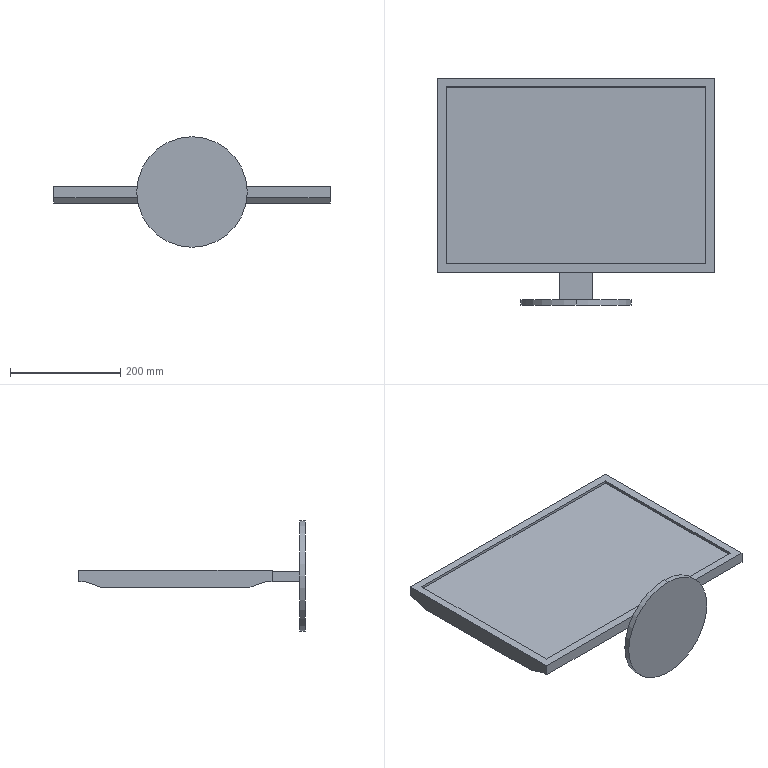Part | SolidWorks | features ICE 4, Extrusion 1 | 1 solid | 22 faces | box 500 x 410 x 200 mm | volume 4616159 mm3 | plane 20 | cylinder 2 | commonest cylinder face diameters 200 x2
STEP:
#1=CARTESIAN_POINT('',(250.,-60.,-90.));
#2=VERTEX_POINT('',#1);
#3=CARTESIAN_POINT('',(250.,-60.,110.));
#4=VERTEX_POINT('',#3);
#5=CARTESIAN_POINT('',(250.,-60.,10.));
#6=DIRECTION('',(0.,-1.,0.));
#7=DIRECTION('',(0.,0.,-1.));
#8=AXIS2_PLACEMENT_3D('',#5,#6,#7);
#9=CIRCLE('',#8,100.);
#10=EDGE_CURVE('',#2,#4,#9,.T.);
#11=ORIENTED_EDGE('',*,*,#10,.F.);
#12=CARTESIAN_POINT('',(250.,-50.,-90.));
#13=VERTEX_POINT('',#12);
#14=CARTESIAN_POINT('',(250.,-60.,-90.));
#15=DIRECTION('',(0.,1.,0.));
#16=VECTOR('',#15,1000.);
#17=LINE('',#14,#16);
#18=EDGE_CURVE('',#2,#13,#17,.T.);
#19=ORIENTED_EDGE('',*,*,#18,.T.);
#20=CARTESIAN_POINT('',(250.,-50.,110.));
#21=VERTEX_POINT('',#20);
#22=CARTESIAN_POINT('',(250.,-50.,10.));
#23=DIRECTION('',(0.,-1.,0.));
#24=DIRECTION('',(0.,0.,-1.));
#25=AXIS2_PLACEMENT_3D('',#22,#23,#24);
#26=CIRCLE('',#25,100.);
#27=EDGE_CURVE('',#13,#21,#26,.T.);
#28=ORIENTED_EDGE('',*,*,#27,.T.);
#29=CARTESIAN_POINT('',(250.,-60.,110.));
#30=DIRECTION('',(0.,1.,0.));
#31=VECTOR('',#30,1000.);
#32=LINE('',#29,#31);
#33=EDGE_CURVE('',#4,#21,#32,.T.);
#34=ORIENTED_EDGE('',*,*,#33,.F.);
#35=EDGE_LOOP('',(#11,#19,#28,#34));
#36=FACE_OUTER_BOUND('',#35,.T.);
#37=CARTESIAN_POINT('',(250.,-60.,10.));
#38=DIRECTION('',(0.,1.,0.));
#39=DIRECTION('',(0.,0.,1.));
#40=AXIS2_PLACEMENT_3D('',#37,#38,#39);
#41=CYLINDRICAL_SURFACE('',#40,100.);
#42=ADVANCED_FACE('',(#36),#41,.T.);
#43=CARTESIAN_POINT('',(280.,0.,0.));
#44=VERTEX_POINT('',#43);
#45=CARTESIAN_POINT('',(280.,0.,18.));
#46=VERTEX_POINT('',#45);
#47=CARTESIAN_POINT('',(280.,0.,18.));
#48=DIRECTION('',(0.,0.,1.));
#49=VECTOR('',#48,1000.);
#50=LINE('',#47,#49);
#51=EDGE_CURVE('',#44,#46,#50,.T.);
#52=ORIENTED_EDGE('',*,*,#51,.F.);
#53=CARTESIAN_POINT('',(500.,0.,0.));
#54=VERTEX_POINT('',#53);
#55=CARTESIAN_POINT('',(0.,0.,0.));
#56=DIRECTION('',(1.,0.,0.));
#57=VECTOR('',#56,1000.);
#58=LINE('',#55,#57);
#59=EDGE_CURVE('',#44,#54,#58,.T.);
#60=ORIENTED_EDGE('',*,*,#59,.T.);
#61=CARTESIAN_POINT('',(500.,0.,20.));
#62=VERTEX_POINT('',#61);
#63=CARTESIAN_POINT('',(500.,0.,20.));
#64=DIRECTION('',(0.,0.,-1.));
#65=VECTOR('',#64,1000.);
#66=LINE('',#63,#65);
#67=EDGE_CURVE('',#62,#54,#66,.T.);
#68=ORIENTED_EDGE('',*,*,#67,.F.);
#69=CARTESIAN_POINT('',(0.,0.,20.));
#70=VERTEX_POINT('',#69);
#71=CARTESIAN_POINT('',(0.,0.,20.));
#72=DIRECTION('',(1.,0.,0.));
#73=VECTOR('',#72,1000.);
#74=LINE('',#71,#73);
#75=EDGE_CURVE('',#70,#62,#74,.T.);
#76=ORIENTED_EDGE('',*,*,#75,.F.);
#77=CARTESIAN_POINT('',(0.,0.,0.));
#78=VERTEX_POINT('',#77);
#79=CARTESIAN_POINT('',(0.,0.,20.));
#80=DIRECTION('',(0.,0.,-1.));
#81=VECTOR('',#80,1000.);
#82=LINE('',#79,#81);
#83=EDGE_CURVE('',#70,#78,#82,.T.);
#84=ORIENTED_EDGE('',*,*,#83,.T.);
#85=CARTESIAN_POINT('',(220.,0.,0.));
#86=VERTEX_POINT('',#85);
#87=CARTESIAN_POINT('',(0.,0.,0.));
#88=DIRECTION('',(1.,0.,0.));
#89=VECTOR('',#88,1000.);
#90=LINE('',#87,#89);
#91=EDGE_CURVE('',#78,#86,#90,.T.);
#92=ORIENTED_EDGE('',*,*,#91,.T.);
#93=CARTESIAN_POINT('',(220.,0.,18.));
#94=VERTEX_POINT('',#93);
#95=CARTESIAN_POINT('',(220.,0.,18.));
#96=DIRECTION('',(0.,0.,-1.));
#97=VECTOR('',#96,1000.);
#98=LINE('',#95,#97);
#99=EDGE_CURVE('',#94,#86,#98,.T.);
#100=ORIENTED_EDGE('',*,*,#99,.F.);
#101=CARTESIAN_POINT('',(220.,0.,18.));
#102=DIRECTION('',(-1.,0.,0.));
#103=VECTOR('',#102,1000.);
#104=LINE('',#101,#103);
#105=EDGE_CURVE('',#46,#94,#104,.T.);
#106=ORIENTED_EDGE('',*,*,#105,.F.);
#107=EDGE_LOOP('',(#52,#60,#68,#76,#84,#92,#100,#106));
#108=FACE_OUTER_BOUND('',#107,.T.);
#109=CARTESIAN_POINT('',(0.,0.,20.));
#110=DIRECTION('',(0.,1.,0.));
#111=DIRECTION('',(0.,0.,1.));
#112=AXIS2_PLACEMENT_3D('',#109,#110,#111);
#113=PLANE('',#112);
#114=ADVANCED_FACE('',(#108),#113,.F.);
#115=CARTESIAN_POINT('',(0.,10.,0.));
#116=VERTEX_POINT('',#115);
#117=CARTESIAN_POINT('',(0.,0.,0.));
#118=DIRECTION('',(0.,-1.,0.));
#119=VECTOR('',#118,1000.);
#120=LINE('',#117,#119);
#121=EDGE_CURVE('',#116,#78,#120,.T.);
#122=ORIENTED_EDGE('',*,*,#121,.F.);
#123=CARTESIAN_POINT('',(500.,10.,0.));
#124=VERTEX_POINT('',#123);
#125=CARTESIAN_POINT('',(0.,10.,0.));
#126=DIRECTION('',(1.,0.,0.));
#127=VECTOR('',#126,1000.);
#128=LINE('',#125,#127);
#129=EDGE_CURVE('',#116,#124,#128,.T.);
#130=ORIENTED_EDGE('',*,*,#129,.T.);
#131=CARTESIAN_POINT('',(500.,0.,0.));
#132=DIRECTION('',(0.,1.,0.));
#133=VECTOR('',#132,1000.);
#134=LINE('',#131,#133);
#135=EDGE_CURVE('',#54,#124,#134,.T.);
#136=ORIENTED_EDGE('',*,*,#135,.F.);
#137=ORIENTED_EDGE('',*,*,#59,.F.);
#138=CARTESIAN_POINT('',(280.,-50.,0.));
#139=VERTEX_POINT('',#138);
#140=CARTESIAN_POINT('',(280.,-50.,0.));
#141=DIRECTION('',(0.,1.,0.));
#142=VECTOR('',#141,1000.);
#143=LINE('',#140,#142);
#144=EDGE_CURVE('',#139,#44,#143,.T.);
#145=ORIENTED_EDGE('',*,*,#144,.F.);
#146=CARTESIAN_POINT('',(220.,-50.,0.));
#147=VERTEX_POINT('',#146);
#148=CARTESIAN_POINT('',(220.,-50.,0.));
#149=DIRECTION('',(1.,0.,0.));
#150=VECTOR('',#149,1000.);
#151=LINE('',#148,#150);
#152=EDGE_CURVE('',#147,#139,#151,.T.);
#153=ORIENTED_EDGE('',*,*,#152,.F.);
#154=CARTESIAN_POINT('',(220.,-50.,0.));
#155=DIRECTION('',(0.,1.,0.));
#156=VECTOR('',#155,1000.);
#157=LINE('',#154,#156);
#158=EDGE_CURVE('',#147,#86,#157,.T.);
#159=ORIENTED_EDGE('',*,*,#158,.T.);
#160=ORIENTED_EDGE('',*,*,#91,.F.);
#161=EDGE_LOOP('',(#122,#130,#136,#137,#145,#153,#159,#160));
#162=FACE_OUTER_BOUND('',#161,.T.);
#163=CARTESIAN_POINT('',(0.,350.,0.));
#164=DIRECTION('',(0.,0.,-1.));
#165=DIRECTION('',(-1.,0.,0.));
#166=AXIS2_PLACEMENT_3D('',#163,#164,#165);
#167=PLANE('',#166);
#168=ADVANCED_FACE('',(#162),#167,.T.);
#169=CARTESIAN_POINT('',(0.,350.,0.));
#170=VERTEX_POINT('',#169);
#171=CARTESIAN_POINT('',(0.,340.,0.));
#172=VERTEX_POINT('',#171);
#173=CARTESIAN_POINT('',(0.,0.,0.));
#174=DIRECTION('',(0.,-1.,0.));
#175=VECTOR('',#174,1000.);
#176=LINE('',#173,#175);
#177=EDGE_CURVE('',#170,#172,#176,.T.);
#178=ORIENTED_EDGE('',*,*,#177,.T.);
#179=CARTESIAN_POINT('',(0.,310.,-10.));
#180=VERTEX_POINT('',#179);
#181=CARTESIAN_POINT('',(0.,310.,-10.));
#182=DIRECTION('',(0.,0.9487,0.3162));
#183=VECTOR('',#182,1000.);
#184=LINE('',#181,#183);
#185=EDGE_CURVE('',#180,#172,#184,.T.);
#186=ORIENTED_EDGE('',*,*,#185,.F.);
#187=CARTESIAN_POINT('',(0.,40.,-10.));
#188=VERTEX_POINT('',#187);
#189=CARTESIAN_POINT('',(0.,40.,-10.));
#190=DIRECTION('',(0.,1.,0.));
#191=VECTOR('',#190,1000.);
#192=LINE('',#189,#191);
#193=EDGE_CURVE('',#188,#180,#192,.T.);
#194=ORIENTED_EDGE('',*,*,#193,.F.);
#195=CARTESIAN_POINT('',(0.,10.,0.));
#196=DIRECTION('',(0.,0.9487,-0.3162));
#197=VECTOR('',#196,1000.);
#198=LINE('',#195,#197);
#199=EDGE_CURVE('',#116,#188,#198,.T.);
#200=ORIENTED_EDGE('',*,*,#199,.F.);
#201=ORIENTED_EDGE('',*,*,#121,.T.);
#202=ORIENTED_EDGE('',*,*,#83,.F.);
#203=CARTESIAN_POINT('',(0.,350.,20.));
#204=VERTEX_POINT('',#203);
#205=CARTESIAN_POINT('',(0.,0.,20.));
#206=DIRECTION('',(0.,-1.,0.));
#207=VECTOR('',#206,1000.);
#208=LINE('',#205,#207);
#209=EDGE_CURVE('',#204,#70,#208,.T.);
#210=ORIENTED_EDGE('',*,*,#209,.F.);
#211=CARTESIAN_POINT('',(0.,350.,20.));
#212=DIRECTION('',(0.,0.,-1.));
#213=VECTOR('',#212,1000.);
#214=LINE('',#211,#213);
#215=EDGE_CURVE('',#204,#170,#214,.T.);
#216=ORIENTED_EDGE('',*,*,#215,.T.);
#217=EDGE_LOOP('',(#178,#186,#194,#200,#201,#202,#210,#216));
#218=FACE_OUTER_BOUND('',#217,.T.);
#219=CARTESIAN_POINT('',(0.,0.,20.));
#220=DIRECTION('',(1.,0.,0.));
#221=DIRECTION('',(0.,0.,-1.));
#222=AXIS2_PLACEMENT_3D('',#219,#220,#221);
#223=PLANE('',#222);
#224=ADVANCED_FACE('',(#218),#223,.F.);
#225=ORIENTED_EDGE('',*,*,#135,.T.);
#226=CARTESIAN_POINT('',(500.,40.,-10.));
#227=VERTEX_POINT('',#226);
#228=CARTESIAN_POINT('',(500.,10.,0.));
#229=DIRECTION('',(0.,0.9487,-0.3162));
#230=VECTOR('',#229,1000.);
#231=LINE('',#228,#230);
#232=EDGE_CURVE('',#124,#227,#231,.T.);
#233=ORIENTED_EDGE('',*,*,#232,.T.);
#234=CARTESIAN_POINT('',(500.,310.,-10.));
#235=VERTEX_POINT('',#234);
#236=CARTESIAN_POINT('',(500.,40.,-10.));
#237=DIRECTION('',(0.,1.,0.));
#238=VECTOR('',#237,1000.);
#239=LINE('',#236,#238);
#240=EDGE_CURVE('',#227,#235,#239,.T.);
#241=ORIENTED_EDGE('',*,*,#240,.T.);
#242=CARTESIAN_POINT('',(500.,340.,0.));
#243=VERTEX_POINT('',#242);
#244=CARTESIAN_POINT('',(500.,310.,-10.));
#245=DIRECTION('',(0.,0.9487,0.3162));
#246=VECTOR('',#245,1000.);
#247=LINE('',#244,#246);
#248=EDGE_CURVE('',#235,#243,#247,.T.);
#249=ORIENTED_EDGE('',*,*,#248,.T.);
#250=CARTESIAN_POINT('',(500.,350.,0.));
#251=VERTEX_POINT('',#250);
#252=CARTESIAN_POINT('',(500.,0.,0.));
#253=DIRECTION('',(0.,1.,0.));
#254=VECTOR('',#253,1000.);
#255=LINE('',#252,#254);
#256=EDGE_CURVE('',#243,#251,#255,.T.);
#257=ORIENTED_EDGE('',*,*,#256,.T.);
#258=CARTESIAN_POINT('',(500.,350.,20.));
#259=VERTEX_POINT('',#258);
#260=CARTESIAN_POINT('',(500.,350.,20.));
#261=DIRECTION('',(0.,0.,-1.));
#262=VECTOR('',#261,1000.);
#263=LINE('',#260,#262);
#264=EDGE_CURVE('',#259,#251,#263,.T.);
#265=ORIENTED_EDGE('',*,*,#264,.F.);
#266=CARTESIAN_POINT('',(500.,0.,20.));
#267=DIRECTION('',(0.,1.,0.));
#268=VECTOR('',#267,1000.);
#269=LINE('',#266,#268);
#270=EDGE_CURVE('',#62,#259,#269,.T.);
#271=ORIENTED_EDGE('',*,*,#270,.F.);
#272=ORIENTED_EDGE('',*,*,#67,.T.);
#273=EDGE_LOOP('',(#225,#233,#241,#249,#257,#265,#271,#272));
#274=FACE_OUTER_BOUND('',#273,.T.);
#275=CARTESIAN_POINT('',(500.,0.,20.));
#276=DIRECTION('',(-1.,0.,0.));
#277=DIRECTION('',(0.,0.,1.));
#278=AXIS2_PLACEMENT_3D('',#275,#276,#277);
#279=PLANE('',#278);
#280=ADVANCED_FACE('',(#274),#279,.F.);
#281=CARTESIAN_POINT('',(0.,350.,0.));
#282=DIRECTION('',(-1.,0.,0.));
#283=VECTOR('',#282,1000.);
#284=LINE('',#281,#283);
#285=EDGE_CURVE('',#251,#170,#284,.T.);
#286=ORIENTED_EDGE('',*,*,#285,.T.);
#287=ORIENTED_EDGE('',*,*,#215,.F.);
#288=CARTESIAN_POINT('',(0.,350.,20.));
#289=DIRECTION('',(-1.,0.,0.));
#290=VECTOR('',#289,1000.);
#291=LINE('',#288,#290);
#292=EDGE_CURVE('',#259,#204,#291,.T.);
#293=ORIENTED_EDGE('',*,*,#292,.F.);
#294=ORIENTED_EDGE('',*,*,#264,.T.);
#295=EDGE_LOOP('',(#286,#287,#293,#294));
#296=FACE_OUTER_BOUND('',#295,.T.);
#297=CARTESIAN_POINT('',(0.,350.,20.));
#298=DIRECTION('',(0.,-1.,0.));
#299=DIRECTION('',(0.,0.,-1.));
#300=AXIS2_PLACEMENT_3D('',#297,#298,#299);
#301=PLANE('',#300);
#302=ADVANCED_FACE('',(#296),#301,.F.);
#303=CARTESIAN_POINT('',(15.,15.,20.));
#304=VERTEX_POINT('',#303);
#305=CARTESIAN_POINT('',(485.,15.,20.));
#306=VERTEX_POINT('',#305);
#307=CARTESIAN_POINT('',(15.,15.,20.));
#308=DIRECTION('',(1.,0.,0.));
#309=VECTOR('',#308,1000.);
#310=LINE('',#307,#309);
#311=EDGE_CURVE('',#304,#306,#310,.T.);
#312=ORIENTED_EDGE('',*,*,#311,.F.);
#313=CARTESIAN_POINT('',(15.,335.,20.));
#314=VERTEX_POINT('',#313);
#315=CARTESIAN_POINT('',(15.,335.,20.));
#316=DIRECTION('',(0.,-1.,0.));
#317=VECTOR('',#316,1000.);
#318=LINE('',#315,#317);
#319=EDGE_CURVE('',#314,#304,#318,.T.);
#320=ORIENTED_EDGE('',*,*,#319,.F.);
#321=CARTESIAN_POINT('',(485.,335.,20.));
#322=VERTEX_POINT('',#321);
#323=CARTESIAN_POINT('',(15.,335.,20.));
#324=DIRECTION('',(-1.,0.,0.));
#325=VECTOR('',#324,1000.);
#326=LINE('',#323,#325);
#327=EDGE_CURVE('',#322,#314,#326,.T.);
#328=ORIENTED_EDGE('',*,*,#327,.F.);
#329=CARTESIAN_POINT('',(485.,335.,20.));
#330=DIRECTION('',(0.,1.,0.));
#331=VECTOR('',#330,1000.);
#332=LINE('',#329,#331);
#333=EDGE_CURVE('',#306,#322,#332,.T.);
#334=ORIENTED_EDGE('',*,*,#333,.F.);
#335=EDGE_LOOP('',(#312,#320,#328,#334));
#336=FACE_BOUND('',#335,.T.);
#337=ORIENTED_EDGE('',*,*,#209,.T.);
#338=ORIENTED_EDGE('',*,*,#75,.T.);
#339=ORIENTED_EDGE('',*,*,#270,.T.);
#340=ORIENTED_EDGE('',*,*,#292,.T.);
#341=EDGE_LOOP('',(#337,#338,#339,#340));
#342=FACE_OUTER_BOUND('',#341,.T.);
#343=CARTESIAN_POINT('',(0.,350.,20.));
#344=DIRECTION('',(0.,0.,-1.));
#345=DIRECTION('',(-1.,0.,0.));
#346=AXIS2_PLACEMENT_3D('',#343,#344,#345);
#347=PLANE('',#346);
#348=ADVANCED_FACE('',(#336,#342),#347,.F.);
#349=CARTESIAN_POINT('',(0.,340.,0.));
#350=DIRECTION('',(1.,0.,0.));
#351=VECTOR('',#350,1000.);
#352=LINE('',#349,#351);
#353=EDGE_CURVE('',#172,#243,#352,.T.);
#354=ORIENTED_EDGE('',*,*,#353,.F.);
#355=ORIENTED_EDGE('',*,*,#177,.F.);
#356=ORIENTED_EDGE('',*,*,#285,.F.);
#357=ORIENTED_EDGE('',*,*,#256,.F.);
#358=EDGE_LOOP('',(#354,#355,#356,#357));
#359=FACE_OUTER_BOUND('',#358,.T.);
#360=CARTESIAN_POINT('',(0.,350.,0.));
#361=DIRECTION('',(0.,0.,-1.));
#362=DIRECTION('',(-1.,0.,0.));
#363=AXIS2_PLACEMENT_3D('',#360,#361,#362);
#364=PLANE('',#363);
#365=ADVANCED_FACE('',(#359),#364,.T.);
#366=ORIENTED_EDGE('',*,*,#248,.F.);
#367=CARTESIAN_POINT('',(0.,310.,-10.));
#368=DIRECTION('',(1.,0.,0.));
#369=VECTOR('',#368,1000.);
#370=LINE('',#367,#369);
#371=EDGE_CURVE('',#180,#235,#370,.T.);
#372=ORIENTED_EDGE('',*,*,#371,.F.);
#373=ORIENTED_EDGE('',*,*,#185,.T.);
#374=ORIENTED_EDGE('',*,*,#353,.T.);
#375=EDGE_LOOP('',(#366,#372,#373,#374));
#376=FACE_OUTER_BOUND('',#375,.T.);
#377=CARTESIAN_POINT('',(0.,310.,-10.));
#378=DIRECTION('',(0.,0.3162,-0.9487));
#379=DIRECTION('',(0.,0.9487,0.3162));
#380=AXIS2_PLACEMENT_3D('',#377,#378,#379);
#381=PLANE('',#380);
#382=ADVANCED_FACE('',(#376),#381,.T.);
#383=ORIENTED_EDGE('',*,*,#240,.F.);
#384=CARTESIAN_POINT('',(0.,40.,-10.));
#385=DIRECTION('',(1.,0.,0.));
#386=VECTOR('',#385,1000.);
#387=LINE('',#384,#386);
#388=EDGE_CURVE('',#188,#227,#387,.T.);
#389=ORIENTED_EDGE('',*,*,#388,.F.);
#390=ORIENTED_EDGE('',*,*,#193,.T.);
#391=ORIENTED_EDGE('',*,*,#371,.T.);
#392=EDGE_LOOP('',(#383,#389,#390,#391));
#393=FACE_OUTER_BOUND('',#392,.T.);
#394=CARTESIAN_POINT('',(0.,40.,-10.));
#395=DIRECTION('',(0.,0.,-1.));
#396=DIRECTION('',(-1.,0.,0.));
#397=AXIS2_PLACEMENT_3D('',#394,#395,#396);
#398=PLANE('',#397);
#399=ADVANCED_FACE('',(#393),#398,.T.);
#400=ORIENTED_EDGE('',*,*,#232,.F.);
#401=ORIENTED_EDGE('',*,*,#129,.F.);
#402=ORIENTED_EDGE('',*,*,#199,.T.);
#403=ORIENTED_EDGE('',*,*,#388,.T.);
#404=EDGE_LOOP('',(#400,#401,#402,#403));
#405=FACE_OUTER_BOUND('',#404,.T.);
#406=CARTESIAN_POINT('',(0.,10.,0.));
#407=DIRECTION('',(0.,-0.3162,-0.9487));
#408=DIRECTION('',(0.,0.9487,-0.3162));
#409=AXIS2_PLACEMENT_3D('',#406,#407,#408);
#410=PLANE('',#409);
#411=ADVANCED_FACE('',(#405),#410,.T.);
#412=ORIENTED_EDGE('',*,*,#319,.T.);
#413=CARTESIAN_POINT('',(15.,15.,15.));
#414=VERTEX_POINT('',#413);
#415=CARTESIAN_POINT('',(15.,15.,15.));
#416=DIRECTION('',(0.,0.,1.));
#417=VECTOR('',#416,1000.);
#418=LINE('',#415,#417);
#419=EDGE_CURVE('',#414,#304,#418,.T.);
#420=ORIENTED_EDGE('',*,*,#419,.F.);
#421=CARTESIAN_POINT('',(15.,335.,15.));
#422=VERTEX_POINT('',#421);
#423=CARTESIAN_POINT('',(15.,335.,15.));
#424=DIRECTION('',(0.,-1.,0.));
#425=VECTOR('',#424,1000.);
#426=LINE('',#423,#425);
#427=EDGE_CURVE('',#422,#414,#426,.T.);
#428=ORIENTED_EDGE('',*,*,#427,.F.);
#429=CARTESIAN_POINT('',(15.,335.,15.));
#430=DIRECTION('',(0.,0.,1.));
#431=VECTOR('',#430,1000.);
#432=LINE('',#429,#431);
#433=EDGE_CURVE('',#422,#314,#432,.T.);
#434=ORIENTED_EDGE('',*,*,#433,.T.);
#435=EDGE_LOOP('',(#412,#420,#428,#434));
#436=FACE_OUTER_BOUND('',#435,.T.);
#437=CARTESIAN_POINT('',(15.,335.,15.));
#438=DIRECTION('',(-1.,0.,0.));
#439=DIRECTION('',(0.,-1.,0.));
#440=AXIS2_PLACEMENT_3D('',#437,#438,#439);
#441=PLANE('',#440);
#442=ADVANCED_FACE('',(#436),#441,.F.);
#443=ORIENTED_EDGE('',*,*,#327,.T.);
#444=ORIENTED_EDGE('',*,*,#433,.F.);
#445=CARTESIAN_POINT('',(485.,335.,15.));
#446=VERTEX_POINT('',#445);
#447=CARTESIAN_POINT('',(15.,335.,15.));
#448=DIRECTION('',(-1.,0.,0.));
#449=VECTOR('',#448,1000.);
#450=LINE('',#447,#449);
#451=EDGE_CURVE('',#446,#422,#450,.T.);
#452=ORIENTED_EDGE('',*,*,#451,.F.);
#453=CARTESIAN_POINT('',(485.,335.,15.));
#454=DIRECTION('',(0.,0.,1.));
#455=VECTOR('',#454,1000.);
#456=LINE('',#453,#455);
#457=EDGE_CURVE('',#446,#322,#456,.T.);
#458=ORIENTED_EDGE('',*,*,#457,.T.);
#459=EDGE_LOOP('',(#443,#444,#452,#458));
#460=FACE_OUTER_BOUND('',#459,.T.);
#461=CARTESIAN_POINT('',(15.,335.,15.));
#462=DIRECTION('',(0.,1.,0.));
#463=DIRECTION('',(0.,0.,1.));
#464=AXIS2_PLACEMENT_3D('',#461,#462,#463);
#465=PLANE('',#464);
#466=ADVANCED_FACE('',(#460),#465,.F.);
#467=ORIENTED_EDGE('',*,*,#333,.T.);
#468=ORIENTED_EDGE('',*,*,#457,.F.);
#469=CARTESIAN_POINT('',(485.,15.,15.));
#470=VERTEX_POINT('',#469);
#471=CARTESIAN_POINT('',(485.,335.,15.));
#472=DIRECTION('',(0.,1.,0.));
#473=VECTOR('',#472,1000.);
#474=LINE('',#471,#473);
#475=EDGE_CURVE('',#470,#446,#474,.T.);
#476=ORIENTED_EDGE('',*,*,#475,.F.);
#477=CARTESIAN_POINT('',(485.,15.,15.));
#478=DIRECTION('',(0.,0.,1.));
#479=VECTOR('',#478,1000.);
#480=LINE('',#477,#479);
#481=EDGE_CURVE('',#470,#306,#480,.T.);
#482=ORIENTED_EDGE('',*,*,#481,.T.);
#483=EDGE_LOOP('',(#467,#468,#476,#482));
#484=FACE_OUTER_BOUND('',#483,.T.);
#485=CARTESIAN_POINT('',(485.,335.,15.));
#486=DIRECTION('',(1.,0.,0.));
#487=DIRECTION('',(0.,1.,0.));
#488=AXIS2_PLACEMENT_3D('',#485,#486,#487);
#489=PLANE('',#488);
#490=ADVANCED_FACE('',(#484),#489,.F.);
#491=ORIENTED_EDGE('',*,*,#311,.T.);
#492=ORIENTED_EDGE('',*,*,#481,.F.);
#493=CARTESIAN_POINT('',(15.,15.,15.));
#494=DIRECTION('',(1.,0.,0.));
#495=VECTOR('',#494,1000.);
#496=LINE('',#493,#495);
#497=EDGE_CURVE('',#414,#470,#496,.T.);
#498=ORIENTED_EDGE('',*,*,#497,.F.);
#499=ORIENTED_EDGE('',*,*,#419,.T.);
#500=EDGE_LOOP('',(#491,#492,#498,#499));
#501=FACE_OUTER_BOUND('',#500,.T.);
#502=CARTESIAN_POINT('',(15.,15.,15.));
#503=DIRECTION('',(0.,-1.,0.));
#504=DIRECTION('',(0.,0.,-1.));
#505=AXIS2_PLACEMENT_3D('',#502,#503,#504);
#506=PLANE('',#505);
#507=ADVANCED_FACE('',(#501),#506,.F.);
#508=ORIENTED_EDGE('',*,*,#427,.T.);
#509=ORIENTED_EDGE('',*,*,#497,.T.);
#510=ORIENTED_EDGE('',*,*,#475,.T.);
#511=ORIENTED_EDGE('',*,*,#451,.T.);
#512=EDGE_LOOP('',(#508,#509,#510,#511));
#513=FACE_OUTER_BOUND('',#512,.T.);
#514=CARTESIAN_POINT('',(15.,15.,15.));
#515=DIRECTION('',(0.,0.,1.));
#516=DIRECTION('',(1.,0.,0.));
#517=AXIS2_PLACEMENT_3D('',#514,#515,#516);
#518=PLANE('',#517);
#519=ADVANCED_FACE('',(#513),#518,.T.);
#520=ORIENTED_EDGE('',*,*,#51,.T.);
#521=CARTESIAN_POINT('',(280.,-50.,18.));
#522=VERTEX_POINT('',#521);
#523=CARTESIAN_POINT('',(280.,-50.,18.));
#524=DIRECTION('',(0.,1.,0.));
#525=VECTOR('',#524,1000.);
#526=LINE('',#523,#525);
#527=EDGE_CURVE('',#522,#46,#526,.T.);
#528=ORIENTED_EDGE('',*,*,#527,.F.);
#529=CARTESIAN_POINT('',(280.,-50.,18.));
#530=DIRECTION('',(0.,0.,1.));
#531=VECTOR('',#530,1000.);
#532=LINE('',#529,#531);
#533=EDGE_CURVE('',#139,#522,#532,.T.);
#534=ORIENTED_EDGE('',*,*,#533,.F.);
#535=ORIENTED_EDGE('',*,*,#144,.T.);
#536=EDGE_LOOP('',(#520,#528,#534,#535));
#537=FACE_OUTER_BOUND('',#536,.T.);
#538=CARTESIAN_POINT('',(280.,-50.,18.));
#539=DIRECTION('',(-1.,0.,0.));
#540=DIRECTION('',(0.,0.,1.));
#541=AXIS2_PLACEMENT_3D('',#538,#539,#540);
#542=PLANE('',#541);
#543=ADVANCED_FACE('',(#537),#542,.F.);
#544=ORIENTED_EDGE('',*,*,#105,.T.);
#545=CARTESIAN_POINT('',(220.,-50.,18.));
#546=VERTEX_POINT('',#545);
#547=CARTESIAN_POINT('',(220.,-50.,18.));
#548=DIRECTION('',(0.,1.,0.));
#549=VECTOR('',#548,1000.);
#550=LINE('',#547,#549);
#551=EDGE_CURVE('',#546,#94,#550,.T.);
#552=ORIENTED_EDGE('',*,*,#551,.F.);
#553=CARTESIAN_POINT('',(220.,-50.,18.));
#554=DIRECTION('',(-1.,0.,0.));
#555=VECTOR('',#554,1000.);
#556=LINE('',#553,#555);
#557=EDGE_CURVE('',#522,#546,#556,.T.);
#558=ORIENTED_EDGE('',*,*,#557,.F.);
#559=ORIENTED_EDGE('',*,*,#527,.T.);
#560=EDGE_LOOP('',(#544,#552,#558,#559));
#561=FACE_OUTER_BOUND('',#560,.T.);
#562=CARTESIAN_POINT('',(220.,-50.,18.));
#563=DIRECTION('',(0.,0.,-1.));
#564=DIRECTION('',(-1.,0.,0.));
#565=AXIS2_PLACEMENT_3D('',#562,#563,#564);
#566=PLANE('',#565);
#567=ADVANCED_FACE('',(#561),#566,.F.);
#568=ORIENTED_EDGE('',*,*,#99,.T.);
#569=ORIENTED_EDGE('',*,*,#158,.F.);
#570=CARTESIAN_POINT('',(220.,-50.,18.));
#571=DIRECTION('',(0.,0.,-1.));
#572=VECTOR('',#571,1000.);
#573=LINE('',#570,#572);
#574=EDGE_CURVE('',#546,#147,#573,.T.);
#575=ORIENTED_EDGE('',*,*,#574,.F.);
#576=ORIENTED_EDGE('',*,*,#551,.T.);
#577=EDGE_LOOP('',(#568,#569,#575,#576));
#578=FACE_OUTER_BOUND('',#577,.T.);
#579=CARTESIAN_POINT('',(220.,-50.,18.));
#580=DIRECTION('',(1.,0.,0.));
#581=DIRECTION('',(0.,0.,-1.));
#582=AXIS2_PLACEMENT_3D('',#579,#580,#581);
#583=PLANE('',#582);
#584=ADVANCED_FACE('',(#578),#583,.F.);
#585=ORIENTED_EDGE('',*,*,#18,.F.);
#586=CARTESIAN_POINT('',(250.,-60.,10.));
#587=DIRECTION('',(0.,-1.,0.));
#588=DIRECTION('',(0.,0.,-1.));
#589=AXIS2_PLACEMENT_3D('',#586,#587,#588);
#590=CIRCLE('',#589,100.);
#591=EDGE_CURVE('',#4,#2,#590,.T.);
#592=ORIENTED_EDGE('',*,*,#591,.F.);
#593=ORIENTED_EDGE('',*,*,#33,.T.);
#594=CARTESIAN_POINT('',(250.,-50.,10.));
#595=DIRECTION('',(0.,-1.,0.));
#596=DIRECTION('',(0.,0.,-1.));
#597=AXIS2_PLACEMENT_3D('',#594,#595,#596);
#598=CIRCLE('',#597,100.);
#599=EDGE_CURVE('',#21,#13,#598,.T.);
#600=ORIENTED_EDGE('',*,*,#599,.T.);
#601=EDGE_LOOP('',(#585,#592,#593,#600));
#602=FACE_OUTER_BOUND('',#601,.T.);
#603=CARTESIAN_POINT('',(250.,-60.,10.));
#604=DIRECTION('',(0.,1.,0.));
#605=DIRECTION('',(0.,0.,1.));
#606=AXIS2_PLACEMENT_3D('',#603,#604,#605);
#607=CYLINDRICAL_SURFACE('',#606,100.);
#608=ADVANCED_FACE('',(#602),#607,.T.);
#609=ORIENTED_EDGE('',*,*,#591,.T.);
#610=ORIENTED_EDGE('',*,*,#10,.T.);
#611=EDGE_LOOP('',(#609,#610));
#612=FACE_OUTER_BOUND('',#611,.T.);
#613=CARTESIAN_POINT('',(250.,-60.,10.));
#614=DIRECTION('',(0.,-1.,0.));
#615=DIRECTION('',(0.,0.,-1.));
#616=AXIS2_PLACEMENT_3D('',#613,#614,#615);
#617=PLANE('',#616);
#618=ADVANCED_FACE('',(#612),#617,.T.);
#619=ORIENTED_EDGE('',*,*,#152,.T.);
#620=ORIENTED_EDGE('',*,*,#533,.T.);
#621=ORIENTED_EDGE('',*,*,#557,.T.);
#622=ORIENTED_EDGE('',*,*,#574,.T.);
#623=EDGE_LOOP('',(#619,#620,#621,#622));
#624=FACE_BOUND('',#623,.T.);
#625=ORIENTED_EDGE('',*,*,#599,.F.);
#626=ORIENTED_EDGE('',*,*,#27,.F.);
#627=EDGE_LOOP('',(#625,#626));
#628=FACE_OUTER_BOUND('',#627,.T.);
#629=CARTESIAN_POINT('',(250.,-50.,10.));
#630=DIRECTION('',(0.,-1.,0.));
#631=DIRECTION('',(0.,0.,-1.));
#632=AXIS2_PLACEMENT_3D('',#629,#630,#631);
#633=PLANE('',#632);
#634=ADVANCED_FACE('',(#624,#628),#633,.F.);
#635=CLOSED_SHELL('',(#42,#114,#168,#224,#280,#302,#348,#365,#382,#399,#411,#442,#466,#490,#507,#519,#543,#567,#584,#608,#618,#634));
#636=MANIFOLD_SOLID_BREP('',#635);
#637=CARTESIAN_POINT('',(0.,0.,0.));
#638=DIRECTION('',(0.,0.,1.));
#639=DIRECTION('',(1.,0.,0.));
#640=AXIS2_PLACEMENT_3D('',#637,#638,#639);
#641=(LENGTH_UNIT()NAMED_UNIT(*)SI_UNIT(.MILLI.,.METRE.));
#642=UNCERTAINTY_MEASURE_WITH_UNIT(LENGTH_MEASURE(0.00001),#641,'','');
#643=(NAMED_UNIT(*)PLANE_ANGLE_UNIT()SI_UNIT($,.RADIAN.));
#644=(NAMED_UNIT(*)SI_UNIT($,.STERADIAN.)SOLID_ANGLE_UNIT());
#645=(GEOMETRIC_REPRESENTATION_CONTEXT(3)GLOBAL_UNCERTAINTY_ASSIGNED_CONTEXT((#642))GLOBAL_UNIT_ASSIGNED_CONTEXT((#641,#643,#644))REPRESENTATION_CONTEXT('',''));
#646=ADVANCED_BREP_SHAPE_REPRESENTATION('',(#636,#640),#645);